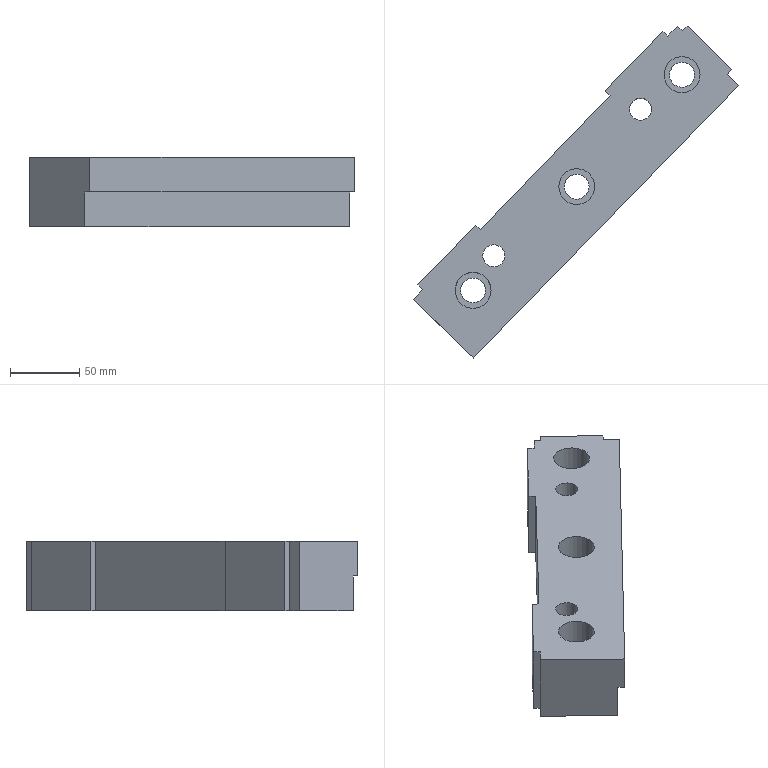Part | NX | features solid 2 | 1 solid | 31 faces | box 235.426 x 240.169 x 50 mm | volume 765936 mm3 | plane 22 | cylinder 8 | spline 1 | commonest cylinder face diameters 18 x3 26 x3 16 x2
STEP:
#1=CARTESIAN_POINT('',(297.563,-516.73,0.));
#2=VERTEX_POINT('',#1);
#3=CARTESIAN_POINT('',(341.291,-558.958,0.));
#4=VERTEX_POINT('',#3);
#5=CARTESIAN_POINT('',(1324.061,-1508.008,-0.000000001));
#6=DIRECTION('',(0.7193,-0.6947,0.));
#7=VECTOR('',#6,1000.);
#8=LINE('',#5,#7);
#9=EDGE_CURVE('',#2,#4,#8,.T.);
#10=ORIENTED_EDGE('',*,*,#9,.T.);
#11=CARTESIAN_POINT('',(532.989,-361.783,0.));
#12=VERTEX_POINT('',#11);
#13=CARTESIAN_POINT('',(119.393,-787.196,0.));
#14=DIRECTION('',(-0.6971,-0.717,0.));
#15=VECTOR('',#14,1000.);
#16=LINE('',#13,#15);
#17=EDGE_CURVE('',#12,#4,#16,.T.);
#18=ORIENTED_EDGE('',*,*,#17,.F.);
#19=CARTESIAN_POINT('',(524.561,-353.645,0.));
#20=VERTEX_POINT('',#19);
#21=CARTESIAN_POINT('',(1002.153,-814.85,0.));
#22=DIRECTION('',(-0.7193,0.6947,0.));
#23=VECTOR('',#22,1000.);
#24=LINE('',#21,#23);
#25=EDGE_CURVE('',#12,#20,#24,.T.);
#26=ORIENTED_EDGE('',*,*,#25,.T.);
#27=CARTESIAN_POINT('',(528.034,-350.048,0.));
#28=VERTEX_POINT('',#27);
#29=CARTESIAN_POINT('',(528.034,-350.048,0.));
#30=DIRECTION('',(0.6947,0.7193,0.));
#31=VECTOR('',#30,1000.);
#32=LINE('',#29,#31);
#33=EDGE_CURVE('',#20,#28,#32,.T.);
#34=ORIENTED_EDGE('',*,*,#33,.T.);
#35=CARTESIAN_POINT('',(495.664,-318.788,0.));
#36=VERTEX_POINT('',#35);
#37=CARTESIAN_POINT('',(484.874,-308.369,0.));
#38=DIRECTION('',(-0.7193,0.6947,0.));
#39=VECTOR('',#38,1000.);
#40=LINE('',#37,#39);
#41=EDGE_CURVE('',#28,#36,#40,.T.);
#42=ORIENTED_EDGE('',*,*,#41,.T.);
#43=CARTESIAN_POINT('',(492.191,-322.385,0.));
#44=VERTEX_POINT('',#43);
#45=CARTESIAN_POINT('',(495.664,-318.788,0.));
#46=DIRECTION('',(0.6947,0.7193,0.));
#47=VECTOR('',#46,1000.);
#48=LINE('',#45,#47);
#49=EDGE_CURVE('',#44,#36,#48,.T.);
#50=ORIENTED_EDGE('',*,*,#49,.F.);
#51=CARTESIAN_POINT('',(488.594,-318.912,0.));
#52=VERTEX_POINT('',#51);
#53=CARTESIAN_POINT('',(1515.092,-1310.189,-0.000000001));
#54=DIRECTION('',(0.7193,-0.6947,0.));
#55=VECTOR('',#54,1000.);
#56=LINE('',#53,#55);
#57=EDGE_CURVE('',#52,#44,#56,.T.);
#58=ORIENTED_EDGE('',*,*,#57,.F.);
#59=CARTESIAN_POINT('',(481.648,-326.105,0.));
#60=VERTEX_POINT('',#59);
#61=CARTESIAN_POINT('',(-977.135,-1836.719,0.));
#62=DIRECTION('',(-0.6947,-0.7193,0.));
#63=VECTOR('',#62,1000.);
#64=LINE('',#61,#63);
#65=EDGE_CURVE('',#52,#60,#64,.T.);
#66=ORIENTED_EDGE('',*,*,#65,.T.);
#67=CARTESIAN_POINT('',(478.051,-322.632,0.));
#68=VERTEX_POINT('',#67);
#69=CARTESIAN_POINT('',(474.454,-319.159,0.));
#70=DIRECTION('',(-0.7193,0.6947,0.));
#71=VECTOR('',#70,1000.);
#72=LINE('',#69,#71);
#73=EDGE_CURVE('',#60,#68,#72,.T.);
#74=ORIENTED_EDGE('',*,*,#73,.T.);
#75=CARTESIAN_POINT('',(436.371,-365.792,0.));
#76=VERTEX_POINT('',#75);
#77=CARTESIAN_POINT('',(488.471,-311.842,0.));
#78=DIRECTION('',(0.6947,0.7193,0.));
#79=VECTOR('',#78,1000.);
#80=LINE('',#77,#79);
#81=EDGE_CURVE('',#76,#68,#80,.T.);
#82=ORIENTED_EDGE('',*,*,#81,.F.);
#83=CARTESIAN_POINT('',(439.968,-369.266,0.));
#84=VERTEX_POINT('',#83);
#85=CARTESIAN_POINT('',(432.775,-362.319,0.));
#86=DIRECTION('',(-0.7193,0.6947,0.));
#87=VECTOR('',#86,1000.);
#88=LINE('',#85,#87);
#89=EDGE_CURVE('',#84,#76,#88,.T.);
#90=ORIENTED_EDGE('',*,*,#89,.F.);
#91=CARTESIAN_POINT('',(346.189,-466.377,0.));
#92=VERTEX_POINT('',#91);
#93=CARTESIAN_POINT('',(-977.135,-1836.719,0.));
#94=DIRECTION('',(-0.6947,-0.7193,0.));
#95=VECTOR('',#94,1000.);
#96=LINE('',#93,#95);
#97=EDGE_CURVE('',#84,#92,#96,.T.);
#98=ORIENTED_EDGE('',*,*,#97,.T.);
#99=CARTESIAN_POINT('',(342.592,-462.903,0.));
#100=VERTEX_POINT('',#99);
#101=CARTESIAN_POINT('',(331.802,-452.483,0.));
#102=DIRECTION('',(0.7193,-0.6947,0.));
#103=VECTOR('',#102,1000.);
#104=LINE('',#101,#103);
#105=EDGE_CURVE('',#100,#92,#104,.T.);
#106=ORIENTED_EDGE('',*,*,#105,.F.);
#107=CARTESIAN_POINT('',(300.913,-506.064,0.));
#108=VERTEX_POINT('',#107);
#109=CARTESIAN_POINT('',(280.073,-527.644,0.));
#110=DIRECTION('',(-0.6947,-0.7193,0.));
#111=VECTOR('',#110,1000.);
#112=LINE('',#109,#111);
#113=EDGE_CURVE('',#100,#108,#112,.T.);
#114=ORIENTED_EDGE('',*,*,#113,.T.);
#115=CARTESIAN_POINT('',(304.51,-509.537,0.));
#116=VERTEX_POINT('',#115);
#117=CARTESIAN_POINT('',(290.123,-495.644,0.));
#118=DIRECTION('',(0.7193,-0.6947,0.));
#119=VECTOR('',#118,1000.);
#120=LINE('',#117,#119);
#121=EDGE_CURVE('',#108,#116,#120,.T.);
#122=ORIENTED_EDGE('',*,*,#121,.T.);
#123=CARTESIAN_POINT('',(-977.135,-1836.719,0.));
#124=DIRECTION('',(-0.6947,-0.7193,0.));
#125=VECTOR('',#124,1000.);
#126=LINE('',#123,#125);
#127=EDGE_CURVE('',#116,#2,#126,.T.);
#128=ORIENTED_EDGE('',*,*,#127,.T.);
#129=EDGE_LOOP('',(#10,#18,#26,#34,#42,#50,#58,#66,#74,#82,#90,#98,#106,#114,#122,#128));
#130=FACE_BOUND('',#129,.T.);
#131=CARTESIAN_POINT('',(428.804,-435.007,0.));
#132=VERTEX_POINT('',#131);
#133=CARTESIAN_POINT('',(415.804,-435.007,0.));
#134=DIRECTION('',(0.,0.,1.));
#135=DIRECTION('',(1.,0.,0.));
#136=AXIS2_PLACEMENT_3D('',#133,#134,#135);
#137=CIRCLE('',#136,13.);
#138=EDGE_CURVE('',#132,#132,#137,.F.);
#139=ORIENTED_EDGE('',*,*,#138,.T.);
#140=EDGE_LOOP('',(#139));
#141=FACE_BOUND('',#140,.T.);
#142=CARTESIAN_POINT('',(363.804,-485.007,0.));
#143=VERTEX_POINT('',#142);
#144=CARTESIAN_POINT('',(355.804,-485.007,0.));
#145=DIRECTION('',(0.,0.,1.));
#146=DIRECTION('',(1.,0.,0.));
#147=AXIS2_PLACEMENT_3D('',#144,#145,#146);
#148=CIRCLE('',#147,8.);
#149=EDGE_CURVE('',#143,#143,#148,.F.);
#150=ORIENTED_EDGE('',*,*,#149,.T.);
#151=EDGE_LOOP('',(#150));
#152=FACE_BOUND('',#151,.T.);
#153=CARTESIAN_POINT('',(470.017,-379.018,0.));
#154=VERTEX_POINT('',#153);
#155=CARTESIAN_POINT('',(462.017,-379.018,0.));
#156=DIRECTION('',(0.,0.,1.));
#157=DIRECTION('',(1.,0.,0.));
#158=AXIS2_PLACEMENT_3D('',#155,#156,#157);
#159=CIRCLE('',#158,8.);
#160=EDGE_CURVE('',#154,#154,#159,.F.);
#161=ORIENTED_EDGE('',*,*,#160,.T.);
#162=EDGE_LOOP('',(#161));
#163=FACE_BOUND('',#162,.T.);
#164=CARTESIAN_POINT('',(505.017,-354.018,0.));
#165=VERTEX_POINT('',#164);
#166=CARTESIAN_POINT('',(492.017,-354.018,0.));
#167=DIRECTION('',(0.,0.,1.));
#168=DIRECTION('',(1.,0.,0.));
#169=AXIS2_PLACEMENT_3D('',#166,#167,#168);
#170=CIRCLE('',#169,13.);
#171=EDGE_CURVE('',#165,#165,#170,.F.);
#172=ORIENTED_EDGE('',*,*,#171,.T.);
#173=EDGE_LOOP('',(#172));
#174=FACE_BOUND('',#173,.T.);
#175=CARTESIAN_POINT('',(353.804,-510.007,0.));
#176=VERTEX_POINT('',#175);
#177=CARTESIAN_POINT('',(340.804,-510.007,0.));
#178=DIRECTION('',(0.,0.,1.));
#179=DIRECTION('',(1.,0.,0.));
#180=AXIS2_PLACEMENT_3D('',#177,#178,#179);
#181=CIRCLE('',#180,13.);
#182=EDGE_CURVE('',#176,#176,#181,.F.);
#183=ORIENTED_EDGE('',*,*,#182,.T.);
#184=EDGE_LOOP('',(#183));
#185=FACE_BOUND('',#184,.T.);
#186=CARTESIAN_POINT('',(484.874,-308.369,0.));
#187=DIRECTION('',(0.,0.,1.));
#188=DIRECTION('',(1.,0.,0.));
#189=AXIS2_PLACEMENT_3D('',#186,#187,#188);
#190=PLANE('',#189);
#191=ADVANCED_FACE('',(#130,#141,#152,#163,#174,#185),#190,.T.);
#192=CARTESIAN_POINT('',(470.017,-379.018,-50.));
#193=VERTEX_POINT('',#192);
#194=CARTESIAN_POINT('',(462.017,-379.018,-50.));
#195=DIRECTION('',(0.,0.,1.));
#196=DIRECTION('',(1.,0.,0.));
#197=AXIS2_PLACEMENT_3D('',#194,#195,#196);
#198=CIRCLE('',#197,8.);
#199=EDGE_CURVE('',#193,#193,#198,.F.);
#200=ORIENTED_EDGE('',*,*,#199,.F.);
#201=EDGE_LOOP('',(#200));
#202=FACE_BOUND('',#201,.T.);
#203=CARTESIAN_POINT('',(363.804,-485.007,-50.));
#204=VERTEX_POINT('',#203);
#205=CARTESIAN_POINT('',(355.804,-485.007,-50.));
#206=DIRECTION('',(0.,0.,1.));
#207=DIRECTION('',(1.,0.,0.));
#208=AXIS2_PLACEMENT_3D('',#205,#206,#207);
#209=CIRCLE('',#208,8.);
#210=EDGE_CURVE('',#204,#204,#209,.F.);
#211=ORIENTED_EDGE('',*,*,#210,.F.);
#212=EDGE_LOOP('',(#211));
#213=FACE_BOUND('',#212,.T.);
#214=CARTESIAN_POINT('',(529.392,-358.31,-50.));
#215=VERTEX_POINT('',#214);
#216=CARTESIAN_POINT('',(337.694,-555.485,-50.));
#217=VERTEX_POINT('',#216);
#218=CARTESIAN_POINT('',(115.808,-783.711,-50.));
#219=DIRECTION('',(-0.6971,-0.717,0.));
#220=VECTOR('',#219,1000.);
#221=LINE('',#218,#220);
#222=EDGE_CURVE('',#215,#217,#221,.T.);
#223=ORIENTED_EDGE('',*,*,#222,.T.);
#224=CARTESIAN_POINT('',(297.563,-516.73,-50.));
#225=VERTEX_POINT('',#224);
#226=CARTESIAN_POINT('',(811.122,-1012.669,-50.));
#227=DIRECTION('',(-0.7193,0.6947,0.));
#228=VECTOR('',#227,1000.);
#229=LINE('',#226,#228);
#230=EDGE_CURVE('',#217,#225,#229,.T.);
#231=ORIENTED_EDGE('',*,*,#230,.T.);
#232=CARTESIAN_POINT('',(304.51,-509.537,-50.));
#233=VERTEX_POINT('',#232);
#234=CARTESIAN_POINT('',(74.905,-747.299,-50.));
#235=DIRECTION('',(0.6947,0.7193,0.));
#236=VECTOR('',#235,1000.);
#237=LINE('',#234,#236);
#238=EDGE_CURVE('',#225,#233,#237,.T.);
#239=ORIENTED_EDGE('',*,*,#238,.T.);
#240=CARTESIAN_POINT('',(300.913,-506.064,-50.));
#241=VERTEX_POINT('',#240);
#242=CARTESIAN_POINT('',(290.123,-495.644,-50.));
#243=DIRECTION('',(-0.7193,0.6947,0.));
#244=VECTOR('',#243,1000.);
#245=LINE('',#242,#244);
#246=EDGE_CURVE('',#233,#241,#245,.T.);
#247=ORIENTED_EDGE('',*,*,#246,.T.);
#248=CARTESIAN_POINT('',(342.592,-462.903,-50.));
#249=VERTEX_POINT('',#248);
#250=CARTESIAN_POINT('',(71.308,-743.826,-50.));
#251=DIRECTION('',(0.6947,0.7193,0.));
#252=VECTOR('',#251,1000.);
#253=LINE('',#250,#252);
#254=EDGE_CURVE('',#241,#249,#253,.T.);
#255=ORIENTED_EDGE('',*,*,#254,.T.);
#256=CARTESIAN_POINT('',(346.189,-466.377,-50.));
#257=VERTEX_POINT('',#256);
#258=CARTESIAN_POINT('',(331.802,-452.483,-50.));
#259=DIRECTION('',(-0.7193,0.6947,0.));
#260=VECTOR('',#259,1000.);
#261=LINE('',#258,#260);
#262=EDGE_CURVE('',#257,#249,#261,.T.);
#263=ORIENTED_EDGE('',*,*,#262,.F.);
#264=CARTESIAN_POINT('',(439.968,-369.266,-50.));
#265=VERTEX_POINT('',#264);
#266=CARTESIAN_POINT('',(74.905,-747.299,-50.));
#267=DIRECTION('',(0.6947,0.7193,0.));
#268=VECTOR('',#267,1000.);
#269=LINE('',#266,#268);
#270=EDGE_CURVE('',#257,#265,#269,.T.);
#271=ORIENTED_EDGE('',*,*,#270,.T.);
#272=CARTESIAN_POINT('',(436.371,-365.792,-50.));
#273=VERTEX_POINT('',#272);
#274=CARTESIAN_POINT('',(425.581,-355.372,-50.));
#275=DIRECTION('',(-0.7193,0.6947,0.));
#276=VECTOR('',#275,1000.);
#277=LINE('',#274,#276);
#278=EDGE_CURVE('',#265,#273,#277,.T.);
#279=ORIENTED_EDGE('',*,*,#278,.T.);
#280=CARTESIAN_POINT('',(478.051,-322.632,-50.));
#281=VERTEX_POINT('',#280);
#282=CARTESIAN_POINT('',(71.308,-743.826,-50.));
#283=DIRECTION('',(0.6947,0.7193,0.));
#284=VECTOR('',#283,1000.);
#285=LINE('',#282,#284);
#286=EDGE_CURVE('',#273,#281,#285,.T.);
#287=ORIENTED_EDGE('',*,*,#286,.T.);
#288=CARTESIAN_POINT('',(481.648,-326.105,-50.));
#289=VERTEX_POINT('',#288);
#290=CARTESIAN_POINT('',(467.261,-312.212,-50.));
#291=DIRECTION('',(-0.7193,0.6947,0.));
#292=VECTOR('',#291,1000.);
#293=LINE('',#290,#292);
#294=EDGE_CURVE('',#289,#281,#293,.T.);
#295=ORIENTED_EDGE('',*,*,#294,.F.);
#296=CARTESIAN_POINT('',(488.594,-318.912,-50.));
#297=VERTEX_POINT('',#296);
#298=CARTESIAN_POINT('',(74.905,-747.299,-50.));
#299=DIRECTION('',(0.6947,0.7193,0.));
#300=VECTOR('',#299,1000.);
#301=LINE('',#298,#300);
#302=EDGE_CURVE('',#289,#297,#301,.T.);
#303=ORIENTED_EDGE('',*,*,#302,.T.);
#304=CARTESIAN_POINT('',(492.191,-322.385,-50.));
#305=VERTEX_POINT('',#304);
#306=CARTESIAN_POINT('',(1002.153,-814.85,-50.));
#307=DIRECTION('',(-0.7193,0.6947,0.));
#308=VECTOR('',#307,1000.);
#309=LINE('',#306,#308);
#310=EDGE_CURVE('',#305,#297,#309,.T.);
#311=ORIENTED_EDGE('',*,*,#310,.F.);
#312=CARTESIAN_POINT('',(495.664,-318.788,-50.));
#313=VERTEX_POINT('',#312);
#314=CARTESIAN_POINT('',(78.502,-750.773,-50.));
#315=DIRECTION('',(0.6947,0.7193,0.));
#316=VECTOR('',#315,1000.);
#317=LINE('',#314,#316);
#318=EDGE_CURVE('',#305,#313,#317,.T.);
#319=ORIENTED_EDGE('',*,*,#318,.T.);
#320=CARTESIAN_POINT('',(528.034,-350.048,-50.));
#321=VERTEX_POINT('',#320);
#322=CARTESIAN_POINT('',(495.664,-318.788,-50.));
#323=DIRECTION('',(0.7193,-0.6947,0.));
#324=VECTOR('',#323,1000.);
#325=LINE('',#322,#324);
#326=EDGE_CURVE('',#321,#313,#325,.F.);
#327=ORIENTED_EDGE('',*,*,#326,.F.);
#328=CARTESIAN_POINT('',(524.561,-353.645,-50.));
#329=VERTEX_POINT('',#328);
#330=CARTESIAN_POINT('',(110.872,-782.032,-50.));
#331=DIRECTION('',(0.6947,0.7193,0.));
#332=VECTOR('',#331,1000.);
#333=LINE('',#330,#332);
#334=EDGE_CURVE('',#329,#321,#333,.T.);
#335=ORIENTED_EDGE('',*,*,#334,.F.);
#336=CARTESIAN_POINT('',(1002.153,-814.85,-50.));
#337=DIRECTION('',(-0.7193,0.6947,0.));
#338=VECTOR('',#337,1000.);
#339=LINE('',#336,#338);
#340=EDGE_CURVE('',#215,#329,#339,.T.);
#341=ORIENTED_EDGE('',*,*,#340,.F.);
#342=EDGE_LOOP('',(#223,#231,#239,#247,#255,#263,#271,#279,#287,#295,#303,#311,#319,#327,#335,#341));
#343=FACE_BOUND('',#342,.T.);
#344=CARTESIAN_POINT('',(349.804,-510.007,-50.));
#345=VERTEX_POINT('',#344);
#346=CARTESIAN_POINT('',(340.804,-510.007,-50.));
#347=DIRECTION('',(0.,0.,1.));
#348=DIRECTION('',(1.,0.,0.));
#349=AXIS2_PLACEMENT_3D('',#346,#347,#348);
#350=CIRCLE('',#349,9.);
#351=EDGE_CURVE('',#345,#345,#350,.F.);
#352=ORIENTED_EDGE('',*,*,#351,.F.);
#353=EDGE_LOOP('',(#352));
#354=FACE_BOUND('',#353,.T.);
#355=CARTESIAN_POINT('',(424.804,-435.007,-50.));
#356=VERTEX_POINT('',#355);
#357=CARTESIAN_POINT('',(415.804,-435.007,-50.));
#358=DIRECTION('',(0.,0.,1.));
#359=DIRECTION('',(1.,0.,0.));
#360=AXIS2_PLACEMENT_3D('',#357,#358,#359);
#361=CIRCLE('',#360,9.);
#362=EDGE_CURVE('',#356,#356,#361,.F.);
#363=ORIENTED_EDGE('',*,*,#362,.F.);
#364=EDGE_LOOP('',(#363));
#365=FACE_BOUND('',#364,.T.);
#366=CARTESIAN_POINT('',(501.017,-354.018,-50.));
#367=VERTEX_POINT('',#366);
#368=CARTESIAN_POINT('',(492.017,-354.018,-50.));
#369=DIRECTION('',(0.,0.,1.));
#370=DIRECTION('',(1.,0.,0.));
#371=AXIS2_PLACEMENT_3D('',#368,#369,#370);
#372=CIRCLE('',#371,9.);
#373=EDGE_CURVE('',#367,#367,#372,.F.);
#374=ORIENTED_EDGE('',*,*,#373,.F.);
#375=EDGE_LOOP('',(#374));
#376=FACE_BOUND('',#375,.T.);
#377=CARTESIAN_POINT('',(588.464,-1243.238,-50.));
#378=DIRECTION('',(0.,0.,1.));
#379=DIRECTION('',(1.,0.,0.));
#380=AXIS2_PLACEMENT_3D('',#377,#378,#379);
#381=PLANE('',#380);
#382=ADVANCED_FACE('',(#202,#213,#343,#354,#365,#376),#381,.F.);
#383=ORIENTED_EDGE('',*,*,#57,.T.);
#384=CARTESIAN_POINT('',(492.191,-322.385,-70.));
#385=DIRECTION('',(0.,0.,-1.));
#386=VECTOR('',#385,1000.);
#387=LINE('',#384,#386);
#388=EDGE_CURVE('',#44,#305,#387,.T.);
#389=ORIENTED_EDGE('',*,*,#388,.T.);
#390=ORIENTED_EDGE('',*,*,#310,.T.);
#391=CARTESIAN_POINT('',(488.594,-318.912,-70.));
#392=DIRECTION('',(0.,0.,1.));
#393=VECTOR('',#392,1000.);
#394=LINE('',#391,#393);
#395=EDGE_CURVE('',#297,#52,#394,.T.);
#396=ORIENTED_EDGE('',*,*,#395,.T.);
#397=EDGE_LOOP('',(#383,#389,#390,#396));
#398=FACE_BOUND('',#397,.T.);
#399=CARTESIAN_POINT('',(1515.092,-1310.189,-70.));
#400=DIRECTION('',(0.6947,0.7193,0.));
#401=DIRECTION('',(-0.7193,0.6947,0.));
#402=AXIS2_PLACEMENT_3D('',#399,#400,#401);
#403=PLANE('',#402);
#404=ADVANCED_FACE('',(#398),#403,.T.);
#405=CARTESIAN_POINT('',(439.968,-369.266,-25.));
#406=DIRECTION('',(0.,0.,-1.));
#407=VECTOR('',#406,1000.);
#408=LINE('',#405,#407);
#409=EDGE_CURVE('',#84,#265,#408,.T.);
#410=ORIENTED_EDGE('',*,*,#409,.T.);
#411=ORIENTED_EDGE('',*,*,#270,.F.);
#412=CARTESIAN_POINT('',(346.189,-466.377,-25.));
#413=DIRECTION('',(0.,0.,-1.));
#414=VECTOR('',#413,1000.);
#415=LINE('',#412,#414);
#416=EDGE_CURVE('',#92,#257,#415,.T.);
#417=ORIENTED_EDGE('',*,*,#416,.F.);
#418=ORIENTED_EDGE('',*,*,#97,.F.);
#419=EDGE_LOOP('',(#410,#411,#417,#418));
#420=FACE_BOUND('',#419,.T.);
#421=CARTESIAN_POINT('',(-977.135,-1836.719,-70.));
#422=DIRECTION('',(0.7193,-0.6947,0.));
#423=DIRECTION('',(0.6947,0.7193,0.));
#424=AXIS2_PLACEMENT_3D('',#421,#422,#423);
#425=PLANE('',#424);
#426=ADVANCED_FACE('',(#420),#425,.F.);
#427=CARTESIAN_POINT('',(304.51,-509.537,-25.));
#428=DIRECTION('',(0.,0.,-1.));
#429=VECTOR('',#428,1000.);
#430=LINE('',#427,#429);
#431=EDGE_CURVE('',#116,#233,#430,.T.);
#432=ORIENTED_EDGE('',*,*,#431,.T.);
#433=ORIENTED_EDGE('',*,*,#238,.F.);
#434=CARTESIAN_POINT('',(297.563,-516.73,-70.));
#435=DIRECTION('',(0.,0.,1.));
#436=VECTOR('',#435,1000.);
#437=LINE('',#434,#436);
#438=EDGE_CURVE('',#225,#2,#437,.T.);
#439=ORIENTED_EDGE('',*,*,#438,.T.);
#440=ORIENTED_EDGE('',*,*,#127,.F.);
#441=EDGE_LOOP('',(#432,#433,#439,#440));
#442=FACE_BOUND('',#441,.T.);
#443=CARTESIAN_POINT('',(-977.135,-1836.719,-70.));
#444=DIRECTION('',(0.7193,-0.6947,0.));
#445=DIRECTION('',(0.6947,0.7193,0.));
#446=AXIS2_PLACEMENT_3D('',#443,#444,#445);
#447=PLANE('',#446);
#448=ADVANCED_FACE('',(#442),#447,.F.);
#449=CARTESIAN_POINT('',(337.694,-555.485,-25.));
#450=VERTEX_POINT('',#449);
#451=CARTESIAN_POINT('',(337.694,-555.485,-70.));
#452=DIRECTION('',(0.,0.,1.));
#453=VECTOR('',#452,1000.);
#454=LINE('',#451,#453);
#455=EDGE_CURVE('',#450,#217,#454,.F.);
#456=ORIENTED_EDGE('',*,*,#455,.T.);
#457=ORIENTED_EDGE('',*,*,#222,.F.);
#458=CARTESIAN_POINT('',(529.392,-358.31,-25.));
#459=VERTEX_POINT('',#458);
#460=CARTESIAN_POINT('',(529.392,-358.31,-70.));
#461=DIRECTION('',(0.,0.,1.));
#462=VECTOR('',#461,1000.);
#463=LINE('',#460,#462);
#464=EDGE_CURVE('',#215,#459,#463,.T.);
#465=ORIENTED_EDGE('',*,*,#464,.T.);
#466=CARTESIAN_POINT('',(529.404,-358.298,-25.));
#467=DIRECTION('',(0.6971,0.717,0.));
#468=VECTOR('',#467,1000.);
#469=LINE('',#466,#468);
#470=EDGE_CURVE('',#450,#459,#469,.T.);
#471=ORIENTED_EDGE('',*,*,#470,.F.);
#472=EDGE_LOOP('',(#456,#457,#465,#471));
#473=FACE_BOUND('',#472,.T.);
#474=CARTESIAN_POINT('',(529.404,-358.298,-70.));
#475=DIRECTION('',(-0.717,0.6971,0.));
#476=DIRECTION('',(-0.6971,-0.717,0.));
#477=AXIS2_PLACEMENT_3D('',#474,#475,#476);
#478=PLANE('',#477);
#479=ADVANCED_FACE('',(#473),#478,.F.);
#480=ORIENTED_EDGE('',*,*,#455,.F.);
#481=CARTESIAN_POINT('',(341.291,-558.958,-25.));
#482=VERTEX_POINT('',#481);
#483=CARTESIAN_POINT('',(341.291,-558.958,-25.));
#484=CARTESIAN_POINT('',(340.092,-557.8,-25.));
#485=CARTESIAN_POINT('',(338.893,-556.642,-25.));
#486=CARTESIAN_POINT('',(337.694,-555.485,-25.));
#487=B_SPLINE_CURVE_WITH_KNOTS('',3,(#483,#484,#485,#486),.UNSPECIFIED.,.F.,.F.,(4,4),(0.,0.005),.UNSPECIFIED.);
#488=EDGE_CURVE('',#482,#450,#487,.T.);
#489=ORIENTED_EDGE('',*,*,#488,.F.);
#490=CARTESIAN_POINT('',(341.291,-558.958,-70.));
#491=DIRECTION('',(0.,0.,1.));
#492=VECTOR('',#491,1000.);
#493=LINE('',#490,#492);
#494=EDGE_CURVE('',#482,#4,#493,.T.);
#495=ORIENTED_EDGE('',*,*,#494,.T.);
#496=ORIENTED_EDGE('',*,*,#9,.F.);
#497=ORIENTED_EDGE('',*,*,#438,.F.);
#498=ORIENTED_EDGE('',*,*,#230,.F.);
#499=EDGE_LOOP('',(#480,#489,#495,#496,#497,#498));
#500=FACE_BOUND('',#499,.T.);
#501=CARTESIAN_POINT('',(1324.061,-1508.008,-70.));
#502=DIRECTION('',(0.6947,0.7193,0.));
#503=DIRECTION('',(-0.7193,0.6947,0.));
#504=AXIS2_PLACEMENT_3D('',#501,#502,#503);
#505=PLANE('',#504);
#506=ADVANCED_FACE('',(#500),#505,.F.);
#507=ORIENTED_EDGE('',*,*,#302,.F.);
#508=CARTESIAN_POINT('',(481.648,-326.105,-25.));
#509=DIRECTION('',(0.,0.,-1.));
#510=VECTOR('',#509,1000.);
#511=LINE('',#508,#510);
#512=EDGE_CURVE('',#60,#289,#511,.T.);
#513=ORIENTED_EDGE('',*,*,#512,.F.);
#514=ORIENTED_EDGE('',*,*,#65,.F.);
#515=ORIENTED_EDGE('',*,*,#395,.F.);
#516=EDGE_LOOP('',(#507,#513,#514,#515));
#517=FACE_BOUND('',#516,.T.);
#518=CARTESIAN_POINT('',(-977.135,-1836.719,-70.));
#519=DIRECTION('',(0.7193,-0.6947,0.));
#520=DIRECTION('',(0.6947,0.7193,0.));
#521=AXIS2_PLACEMENT_3D('',#518,#519,#520);
#522=PLANE('',#521);
#523=ADVANCED_FACE('',(#517),#522,.F.);
#524=CARTESIAN_POINT('',(532.989,-361.783,-25.));
#525=VERTEX_POINT('',#524);
#526=CARTESIAN_POINT('',(532.989,-361.783,-25.));
#527=CARTESIAN_POINT('',(531.79,-360.625,-25.));
#528=CARTESIAN_POINT('',(530.591,-359.468,-25.));
#529=CARTESIAN_POINT('',(529.392,-358.31,-25.));
#530=B_SPLINE_CURVE_WITH_KNOTS('',3,(#526,#527,#528,#529),.UNSPECIFIED.,.F.,.F.,(4,4),(0.03993,0.04493),.UNSPECIFIED.);
#531=EDGE_CURVE('',#525,#459,#530,.T.);
#532=ORIENTED_EDGE('',*,*,#531,.T.);
#533=ORIENTED_EDGE('',*,*,#464,.F.);
#534=ORIENTED_EDGE('',*,*,#340,.T.);
#535=CARTESIAN_POINT('',(524.561,-353.645,-70.));
#536=DIRECTION('',(0.,0.,-1.));
#537=VECTOR('',#536,1000.);
#538=LINE('',#535,#537);
#539=EDGE_CURVE('',#20,#329,#538,.T.);
#540=ORIENTED_EDGE('',*,*,#539,.F.);
#541=ORIENTED_EDGE('',*,*,#25,.F.);
#542=CARTESIAN_POINT('',(532.989,-361.783,-70.));
#543=DIRECTION('',(0.,0.,1.));
#544=VECTOR('',#543,1000.);
#545=LINE('',#542,#544);
#546=EDGE_CURVE('',#525,#12,#545,.T.);
#547=ORIENTED_EDGE('',*,*,#546,.F.);
#548=EDGE_LOOP('',(#532,#533,#534,#540,#541,#547));
#549=FACE_BOUND('',#548,.T.);
#550=CARTESIAN_POINT('',(1515.092,-1310.189,-70.));
#551=DIRECTION('',(0.6947,0.7193,0.));
#552=DIRECTION('',(-0.7193,0.6947,0.));
#553=AXIS2_PLACEMENT_3D('',#550,#551,#552);
#554=PLANE('',#553);
#555=ADVANCED_FACE('',(#549),#554,.T.);
#556=CARTESIAN_POINT('',(342.592,-462.903,-25.));
#557=DIRECTION('',(0.,0.,-1.));
#558=VECTOR('',#557,1000.);
#559=LINE('',#556,#558);
#560=EDGE_CURVE('',#100,#249,#559,.T.);
#561=ORIENTED_EDGE('',*,*,#560,.F.);
#562=ORIENTED_EDGE('',*,*,#105,.T.);
#563=ORIENTED_EDGE('',*,*,#416,.T.);
#564=ORIENTED_EDGE('',*,*,#262,.T.);
#565=EDGE_LOOP('',(#561,#562,#563,#564));
#566=FACE_BOUND('',#565,.T.);
#567=CARTESIAN_POINT('',(331.802,-452.483,-25.));
#568=DIRECTION('',(0.6947,0.7193,0.));
#569=DIRECTION('',(-0.7193,0.6947,0.));
#570=AXIS2_PLACEMENT_3D('',#567,#568,#569);
#571=PLANE('',#570);
#572=ADVANCED_FACE('',(#566),#571,.T.);
#573=ORIENTED_EDGE('',*,*,#121,.F.);
#574=CARTESIAN_POINT('',(300.913,-506.064,-25.));
#575=DIRECTION('',(0.,0.,-1.));
#576=VECTOR('',#575,1000.);
#577=LINE('',#574,#576);
#578=EDGE_CURVE('',#108,#241,#577,.T.);
#579=ORIENTED_EDGE('',*,*,#578,.T.);
#580=ORIENTED_EDGE('',*,*,#246,.F.);
#581=ORIENTED_EDGE('',*,*,#431,.F.);
#582=EDGE_LOOP('',(#573,#579,#580,#581));
#583=FACE_BOUND('',#582,.T.);
#584=CARTESIAN_POINT('',(290.123,-495.644,-25.));
#585=DIRECTION('',(0.6947,0.7193,0.));
#586=DIRECTION('',(-0.7193,0.6947,0.));
#587=AXIS2_PLACEMENT_3D('',#584,#585,#586);
#588=PLANE('',#587);
#589=ADVANCED_FACE('',(#583),#588,.F.);
#590=ORIENTED_EDGE('',*,*,#113,.F.);
#591=ORIENTED_EDGE('',*,*,#560,.T.);
#592=ORIENTED_EDGE('',*,*,#254,.F.);
#593=ORIENTED_EDGE('',*,*,#578,.F.);
#594=EDGE_LOOP('',(#590,#591,#592,#593));
#595=FACE_BOUND('',#594,.T.);
#596=CARTESIAN_POINT('',(280.073,-527.644,-25.));
#597=DIRECTION('',(0.7193,-0.6947,0.));
#598=DIRECTION('',(0.,0.,-1.));
#599=AXIS2_PLACEMENT_3D('',#596,#597,#598);
#600=PLANE('',#599);
#601=ADVANCED_FACE('',(#595),#600,.F.);
#602=ORIENTED_EDGE('',*,*,#73,.F.);
#603=ORIENTED_EDGE('',*,*,#512,.T.);
#604=ORIENTED_EDGE('',*,*,#294,.T.);
#605=CARTESIAN_POINT('',(478.051,-322.632,-25.));
#606=DIRECTION('',(0.,0.,-1.));
#607=VECTOR('',#606,1000.);
#608=LINE('',#605,#607);
#609=EDGE_CURVE('',#68,#281,#608,.T.);
#610=ORIENTED_EDGE('',*,*,#609,.F.);
#611=EDGE_LOOP('',(#602,#603,#604,#610));
#612=FACE_BOUND('',#611,.T.);
#613=CARTESIAN_POINT('',(467.261,-312.212,-25.));
#614=DIRECTION('',(0.6947,0.7193,0.));
#615=DIRECTION('',(-0.7193,0.6947,0.));
#616=AXIS2_PLACEMENT_3D('',#613,#614,#615);
#617=PLANE('',#616);
#618=ADVANCED_FACE('',(#612),#617,.T.);
#619=ORIENTED_EDGE('',*,*,#409,.F.);
#620=ORIENTED_EDGE('',*,*,#89,.T.);
#621=CARTESIAN_POINT('',(436.371,-365.792,-25.));
#622=DIRECTION('',(0.,0.,-1.));
#623=VECTOR('',#622,1000.);
#624=LINE('',#621,#623);
#625=EDGE_CURVE('',#76,#273,#624,.T.);
#626=ORIENTED_EDGE('',*,*,#625,.T.);
#627=ORIENTED_EDGE('',*,*,#278,.F.);
#628=EDGE_LOOP('',(#619,#620,#626,#627));
#629=FACE_BOUND('',#628,.T.);
#630=CARTESIAN_POINT('',(425.581,-355.372,-25.));
#631=DIRECTION('',(0.6947,0.7193,0.));
#632=DIRECTION('',(-0.7193,0.6947,0.));
#633=AXIS2_PLACEMENT_3D('',#630,#631,#632);
#634=PLANE('',#633);
#635=ADVANCED_FACE('',(#629),#634,.F.);
#636=ORIENTED_EDGE('',*,*,#625,.F.);
#637=ORIENTED_EDGE('',*,*,#81,.T.);
#638=ORIENTED_EDGE('',*,*,#609,.T.);
#639=ORIENTED_EDGE('',*,*,#286,.F.);
#640=EDGE_LOOP('',(#636,#637,#638,#639));
#641=FACE_BOUND('',#640,.T.);
#642=CARTESIAN_POINT('',(436.371,-365.792,-25.));
#643=DIRECTION('',(0.7193,-0.6947,0.));
#644=DIRECTION('',(0.,0.,-1.));
#645=AXIS2_PLACEMENT_3D('',#642,#643,#644);
#646=PLANE('',#645);
#647=ADVANCED_FACE('',(#641),#646,.F.);
#648=CARTESIAN_POINT('',(495.664,-318.788,-25.));
#649=DIRECTION('',(0.,0.,-1.));
#650=VECTOR('',#649,1000.);
#651=LINE('',#648,#650);
#652=EDGE_CURVE('',#36,#313,#651,.T.);
#653=ORIENTED_EDGE('',*,*,#652,.T.);
#654=ORIENTED_EDGE('',*,*,#318,.F.);
#655=ORIENTED_EDGE('',*,*,#388,.F.);
#656=ORIENTED_EDGE('',*,*,#49,.T.);
#657=EDGE_LOOP('',(#653,#654,#655,#656));
#658=FACE_BOUND('',#657,.T.);
#659=CARTESIAN_POINT('',(492.191,-322.385,-25.));
#660=DIRECTION('',(0.7193,-0.6947,0.));
#661=DIRECTION('',(0.6947,0.7193,0.));
#662=AXIS2_PLACEMENT_3D('',#659,#660,#661);
#663=PLANE('',#662);
#664=ADVANCED_FACE('',(#658),#663,.F.);
#665=CARTESIAN_POINT('',(528.034,-350.048,-25.));
#666=DIRECTION('',(0.,0.,-1.));
#667=VECTOR('',#666,1000.);
#668=LINE('',#665,#667);
#669=EDGE_CURVE('',#28,#321,#668,.T.);
#670=ORIENTED_EDGE('',*,*,#669,.F.);
#671=ORIENTED_EDGE('',*,*,#33,.F.);
#672=ORIENTED_EDGE('',*,*,#539,.T.);
#673=ORIENTED_EDGE('',*,*,#334,.T.);
#674=EDGE_LOOP('',(#670,#671,#672,#673));
#675=FACE_BOUND('',#674,.T.);
#676=CARTESIAN_POINT('',(524.561,-353.645,-25.));
#677=DIRECTION('',(0.7193,-0.6947,0.));
#678=DIRECTION('',(0.6947,0.7193,0.));
#679=AXIS2_PLACEMENT_3D('',#676,#677,#678);
#680=PLANE('',#679);
#681=ADVANCED_FACE('',(#675),#680,.T.);
#682=ORIENTED_EDGE('',*,*,#652,.F.);
#683=ORIENTED_EDGE('',*,*,#41,.F.);
#684=ORIENTED_EDGE('',*,*,#669,.T.);
#685=ORIENTED_EDGE('',*,*,#326,.T.);
#686=EDGE_LOOP('',(#682,#683,#684,#685));
#687=FACE_BOUND('',#686,.T.);
#688=CARTESIAN_POINT('',(495.664,-318.788,-25.));
#689=DIRECTION('',(0.6947,0.7193,0.));
#690=DIRECTION('',(0.,0.,-1.));
#691=AXIS2_PLACEMENT_3D('',#688,#689,#690);
#692=PLANE('',#691);
#693=ADVANCED_FACE('',(#687),#692,.T.);
#694=CARTESIAN_POINT('',(532.989,-361.783,-25.));
#695=CARTESIAN_POINT('',(469.089,-427.508,-25.));
#696=CARTESIAN_POINT('',(405.19,-493.233,-25.));
#697=CARTESIAN_POINT('',(341.291,-558.958,-25.));
#698=B_SPLINE_CURVE_WITH_KNOTS('',3,(#694,#695,#696,#697),.UNSPECIFIED.,.F.,.F.,(4,4),(0.4325,0.7075),.UNSPECIFIED.);
#699=EDGE_CURVE('',#525,#482,#698,.T.);
#700=ORIENTED_EDGE('',*,*,#699,.F.);
#701=ORIENTED_EDGE('',*,*,#546,.T.);
#702=ORIENTED_EDGE('',*,*,#17,.T.);
#703=ORIENTED_EDGE('',*,*,#494,.F.);
#704=EDGE_LOOP('',(#700,#701,#702,#703));
#705=FACE_BOUND('',#704,.T.);
#706=CARTESIAN_POINT('',(532.989,-361.783,-70.));
#707=DIRECTION('',(-0.717,0.6971,0.));
#708=DIRECTION('',(-0.6971,-0.717,0.));
#709=AXIS2_PLACEMENT_3D('',#706,#707,#708);
#710=PLANE('',#709);
#711=ADVANCED_FACE('',(#705),#710,.F.);
#712=ORIENTED_EDGE('',*,*,#699,.T.);
#713=ORIENTED_EDGE('',*,*,#488,.T.);
#714=ORIENTED_EDGE('',*,*,#470,.T.);
#715=ORIENTED_EDGE('',*,*,#531,.F.);
#716=EDGE_LOOP('',(#712,#713,#714,#715));
#717=FACE_BOUND('',#716,.T.);
#718=CARTESIAN_POINT('',(534.21,-360.527,-25.));
#719=CARTESIAN_POINT('',(530.625,-357.042,-25.));
#720=CARTESIAN_POINT('',(525.628,-369.354,-25.));
#721=CARTESIAN_POINT('',(522.043,-365.868,-25.));
#722=CARTESIAN_POINT('',(508.79,-386.673,-25.));
#723=CARTESIAN_POINT('',(505.205,-383.188,-25.));
#724=CARTESIAN_POINT('',(476.327,-420.063,-25.));
#725=CARTESIAN_POINT('',(472.742,-416.578,-25.));
#726=CARTESIAN_POINT('',(437.169,-460.341,-25.));
#727=CARTESIAN_POINT('',(433.584,-456.855,-25.));
#728=CARTESIAN_POINT('',(397.997,-500.632,-25.));
#729=CARTESIAN_POINT('',(394.412,-497.147,-25.));
#730=CARTESIAN_POINT('',(365.507,-534.05,-25.));
#731=CARTESIAN_POINT('',(361.922,-530.565,-25.));
#732=CARTESIAN_POINT('',(348.649,-551.39,-25.));
#733=CARTESIAN_POINT('',(345.064,-547.905,-25.));
#734=CARTESIAN_POINT('',(340.057,-560.227,-25.));
#735=CARTESIAN_POINT('',(336.472,-556.742,-25.));
#736=B_SPLINE_SURFACE_WITH_KNOTS('',3,1,((#718,#719),(#720,#721),(#722,#723),(#724,#725),(#726,#727),(#728,#729),(#730,#731),(#732,#733),(#734,#735)),.SURF_OF_LINEAR_EXTRUSION.,.F.,.F.,.F.,(4,1,1,1,1,1,4),(2,2),(-0.006,0.1205,0.247,0.5,0.753,0.8796,1.006),(0.,1.),.UNSPECIFIED.);
#737=ADVANCED_FACE('',(#717),#736,.T.);
#738=CARTESIAN_POINT('',(331.804,-510.007,-30.));
#739=VERTEX_POINT('',#738);
#740=CARTESIAN_POINT('',(340.804,-510.007,-30.));
#741=DIRECTION('',(0.,0.,-1.));
#742=DIRECTION('',(-1.,0.,0.));
#743=AXIS2_PLACEMENT_3D('',#740,#741,#742);
#744=CIRCLE('',#743,9.);
#745=EDGE_CURVE('',#739,#739,#744,.T.);
#746=ORIENTED_EDGE('',*,*,#745,.F.);
#747=EDGE_LOOP('',(#746));
#748=FACE_BOUND('',#747,.T.);
#749=ORIENTED_EDGE('',*,*,#351,.T.);
#750=EDGE_LOOP('',(#749));
#751=FACE_BOUND('',#750,.T.);
#752=CARTESIAN_POINT('',(340.804,-510.007,-125.));
#753=DIRECTION('',(0.,0.,1.));
#754=DIRECTION('',(1.,0.,0.));
#755=AXIS2_PLACEMENT_3D('',#752,#753,#754);
#756=CYLINDRICAL_SURFACE('',#755,9.);
#757=ADVANCED_FACE('',(#748,#751),#756,.F.);
#758=ORIENTED_EDGE('',*,*,#149,.F.);
#759=EDGE_LOOP('',(#758));
#760=FACE_BOUND('',#759,.T.);
#761=ORIENTED_EDGE('',*,*,#210,.T.);
#762=EDGE_LOOP('',(#761));
#763=FACE_BOUND('',#762,.T.);
#764=CARTESIAN_POINT('',(355.804,-485.007,-125.));
#765=DIRECTION('',(0.,0.,1.));
#766=DIRECTION('',(1.,0.,0.));
#767=AXIS2_PLACEMENT_3D('',#764,#765,#766);
#768=CYLINDRICAL_SURFACE('',#767,8.);
#769=ADVANCED_FACE('',(#760,#763),#768,.F.);
#770=CARTESIAN_POINT('',(406.804,-435.007,-30.));
#771=VERTEX_POINT('',#770);
#772=CARTESIAN_POINT('',(415.804,-435.007,-30.));
#773=DIRECTION('',(0.,0.,-1.));
#774=DIRECTION('',(-1.,0.,0.));
#775=AXIS2_PLACEMENT_3D('',#772,#773,#774);
#776=CIRCLE('',#775,9.);
#777=EDGE_CURVE('',#771,#771,#776,.T.);
#778=ORIENTED_EDGE('',*,*,#777,.F.);
#779=EDGE_LOOP('',(#778));
#780=FACE_BOUND('',#779,.T.);
#781=ORIENTED_EDGE('',*,*,#362,.T.);
#782=EDGE_LOOP('',(#781));
#783=FACE_BOUND('',#782,.T.);
#784=CARTESIAN_POINT('',(415.804,-435.007,-125.));
#785=DIRECTION('',(0.,0.,1.));
#786=DIRECTION('',(1.,0.,0.));
#787=AXIS2_PLACEMENT_3D('',#784,#785,#786);
#788=CYLINDRICAL_SURFACE('',#787,9.);
#789=ADVANCED_FACE('',(#780,#783),#788,.F.);
#790=ORIENTED_EDGE('',*,*,#160,.F.);
#791=EDGE_LOOP('',(#790));
#792=FACE_BOUND('',#791,.T.);
#793=ORIENTED_EDGE('',*,*,#199,.T.);
#794=EDGE_LOOP('',(#793));
#795=FACE_BOUND('',#794,.T.);
#796=CARTESIAN_POINT('',(462.017,-379.018,-125.));
#797=DIRECTION('',(0.,0.,1.));
#798=DIRECTION('',(1.,0.,0.));
#799=AXIS2_PLACEMENT_3D('',#796,#797,#798);
#800=CYLINDRICAL_SURFACE('',#799,8.);
#801=ADVANCED_FACE('',(#792,#795),#800,.F.);
#802=CARTESIAN_POINT('',(483.017,-354.018,-30.));
#803=VERTEX_POINT('',#802);
#804=CARTESIAN_POINT('',(492.017,-354.018,-30.));
#805=DIRECTION('',(0.,0.,-1.));
#806=DIRECTION('',(-1.,0.,0.));
#807=AXIS2_PLACEMENT_3D('',#804,#805,#806);
#808=CIRCLE('',#807,9.);
#809=EDGE_CURVE('',#803,#803,#808,.T.);
#810=ORIENTED_EDGE('',*,*,#809,.F.);
#811=EDGE_LOOP('',(#810));
#812=FACE_BOUND('',#811,.T.);
#813=ORIENTED_EDGE('',*,*,#373,.T.);
#814=EDGE_LOOP('',(#813));
#815=FACE_BOUND('',#814,.T.);
#816=CARTESIAN_POINT('',(492.017,-354.018,-125.));
#817=DIRECTION('',(0.,0.,1.));
#818=DIRECTION('',(1.,0.,0.));
#819=AXIS2_PLACEMENT_3D('',#816,#817,#818);
#820=CYLINDRICAL_SURFACE('',#819,9.);
#821=ADVANCED_FACE('',(#812,#815),#820,.F.);
#822=CARTESIAN_POINT('',(505.017,-354.018,-30.));
#823=VERTEX_POINT('',#822);
#824=CARTESIAN_POINT('',(492.017,-354.018,-30.));
#825=DIRECTION('',(0.,0.,-1.));
#826=DIRECTION('',(1.,0.,0.));
#827=AXIS2_PLACEMENT_3D('',#824,#825,#826);
#828=CIRCLE('',#827,13.);
#829=EDGE_CURVE('',#823,#823,#828,.T.);
#830=ORIENTED_EDGE('',*,*,#829,.T.);
#831=EDGE_LOOP('',(#830));
#832=FACE_BOUND('',#831,.T.);
#833=ORIENTED_EDGE('',*,*,#171,.F.);
#834=EDGE_LOOP('',(#833));
#835=FACE_BOUND('',#834,.T.);
#836=CARTESIAN_POINT('',(492.017,-354.018,-30.));
#837=DIRECTION('',(0.,0.,1.));
#838=DIRECTION('',(1.,0.,0.));
#839=AXIS2_PLACEMENT_3D('',#836,#837,#838);
#840=CYLINDRICAL_SURFACE('',#839,13.);
#841=ADVANCED_FACE('',(#832,#835),#840,.F.);
#842=ORIENTED_EDGE('',*,*,#809,.T.);
#843=EDGE_LOOP('',(#842));
#844=FACE_BOUND('',#843,.T.);
#845=ORIENTED_EDGE('',*,*,#829,.F.);
#846=EDGE_LOOP('',(#845));
#847=FACE_BOUND('',#846,.T.);
#848=CARTESIAN_POINT('',(492.017,-354.018,-30.));
#849=DIRECTION('',(0.,0.,-1.));
#850=DIRECTION('',(-1.,0.,0.));
#851=AXIS2_PLACEMENT_3D('',#848,#849,#850);
#852=PLANE('',#851);
#853=ADVANCED_FACE('',(#844,#847),#852,.F.);
#854=CARTESIAN_POINT('',(428.804,-435.007,-30.));
#855=VERTEX_POINT('',#854);
#856=CARTESIAN_POINT('',(415.804,-435.007,-30.));
#857=DIRECTION('',(0.,0.,-1.));
#858=DIRECTION('',(1.,0.,0.));
#859=AXIS2_PLACEMENT_3D('',#856,#857,#858);
#860=CIRCLE('',#859,13.);
#861=EDGE_CURVE('',#855,#855,#860,.T.);
#862=ORIENTED_EDGE('',*,*,#861,.T.);
#863=EDGE_LOOP('',(#862));
#864=FACE_BOUND('',#863,.T.);
#865=ORIENTED_EDGE('',*,*,#138,.F.);
#866=EDGE_LOOP('',(#865));
#867=FACE_BOUND('',#866,.T.);
#868=CARTESIAN_POINT('',(415.804,-435.007,-30.));
#869=DIRECTION('',(0.,0.,1.));
#870=DIRECTION('',(1.,0.,0.));
#871=AXIS2_PLACEMENT_3D('',#868,#869,#870);
#872=CYLINDRICAL_SURFACE('',#871,13.);
#873=ADVANCED_FACE('',(#864,#867),#872,.F.);
#874=ORIENTED_EDGE('',*,*,#777,.T.);
#875=EDGE_LOOP('',(#874));
#876=FACE_BOUND('',#875,.T.);
#877=ORIENTED_EDGE('',*,*,#861,.F.);
#878=EDGE_LOOP('',(#877));
#879=FACE_BOUND('',#878,.T.);
#880=CARTESIAN_POINT('',(415.804,-435.007,-30.));
#881=DIRECTION('',(0.,0.,-1.));
#882=DIRECTION('',(-1.,0.,0.));
#883=AXIS2_PLACEMENT_3D('',#880,#881,#882);
#884=PLANE('',#883);
#885=ADVANCED_FACE('',(#876,#879),#884,.F.);
#886=CARTESIAN_POINT('',(353.804,-510.007,-30.));
#887=VERTEX_POINT('',#886);
#888=CARTESIAN_POINT('',(340.804,-510.007,-30.));
#889=DIRECTION('',(0.,0.,-1.));
#890=DIRECTION('',(1.,0.,0.));
#891=AXIS2_PLACEMENT_3D('',#888,#889,#890);
#892=CIRCLE('',#891,13.);
#893=EDGE_CURVE('',#887,#887,#892,.T.);
#894=ORIENTED_EDGE('',*,*,#893,.T.);
#895=EDGE_LOOP('',(#894));
#896=FACE_BOUND('',#895,.T.);
#897=ORIENTED_EDGE('',*,*,#182,.F.);
#898=EDGE_LOOP('',(#897));
#899=FACE_BOUND('',#898,.T.);
#900=CARTESIAN_POINT('',(340.804,-510.007,-30.));
#901=DIRECTION('',(0.,0.,1.));
#902=DIRECTION('',(1.,0.,0.));
#903=AXIS2_PLACEMENT_3D('',#900,#901,#902);
#904=CYLINDRICAL_SURFACE('',#903,13.);
#905=ADVANCED_FACE('',(#896,#899),#904,.F.);
#906=ORIENTED_EDGE('',*,*,#745,.T.);
#907=EDGE_LOOP('',(#906));
#908=FACE_BOUND('',#907,.T.);
#909=ORIENTED_EDGE('',*,*,#893,.F.);
#910=EDGE_LOOP('',(#909));
#911=FACE_BOUND('',#910,.T.);
#912=CARTESIAN_POINT('',(340.804,-510.007,-30.));
#913=DIRECTION('',(0.,0.,-1.));
#914=DIRECTION('',(-1.,0.,0.));
#915=AXIS2_PLACEMENT_3D('',#912,#913,#914);
#916=PLANE('',#915);
#917=ADVANCED_FACE('',(#908,#911),#916,.F.);
#918=CLOSED_SHELL('',(#191,#382,#404,#426,#448,#479,#506,#523,#555,#572,#589,#601,#618,#635,#647,#664,#681,#693,#711,#737,#757,#769,#789,#801,#821,#841,#853,#873,#885,#905,#917));
#919=MANIFOLD_SOLID_BREP('',#918);
#920=(LENGTH_UNIT()NAMED_UNIT(*)SI_UNIT(.MILLI.,.METRE.));
#921=UNCERTAINTY_MEASURE_WITH_UNIT(LENGTH_MEASURE(0.0508),#920,'','');
#922=(NAMED_UNIT(*)PLANE_ANGLE_UNIT()SI_UNIT($,.RADIAN.));
#923=(NAMED_UNIT(*)SI_UNIT($,.STERADIAN.)SOLID_ANGLE_UNIT());
#924=(GEOMETRIC_REPRESENTATION_CONTEXT(3)GLOBAL_UNCERTAINTY_ASSIGNED_CONTEXT((#921))GLOBAL_UNIT_ASSIGNED_CONTEXT((#920,#922,#923))REPRESENTATION_CONTEXT('',''));
#925=ADVANCED_BREP_SHAPE_REPRESENTATION('',(#919),#924);